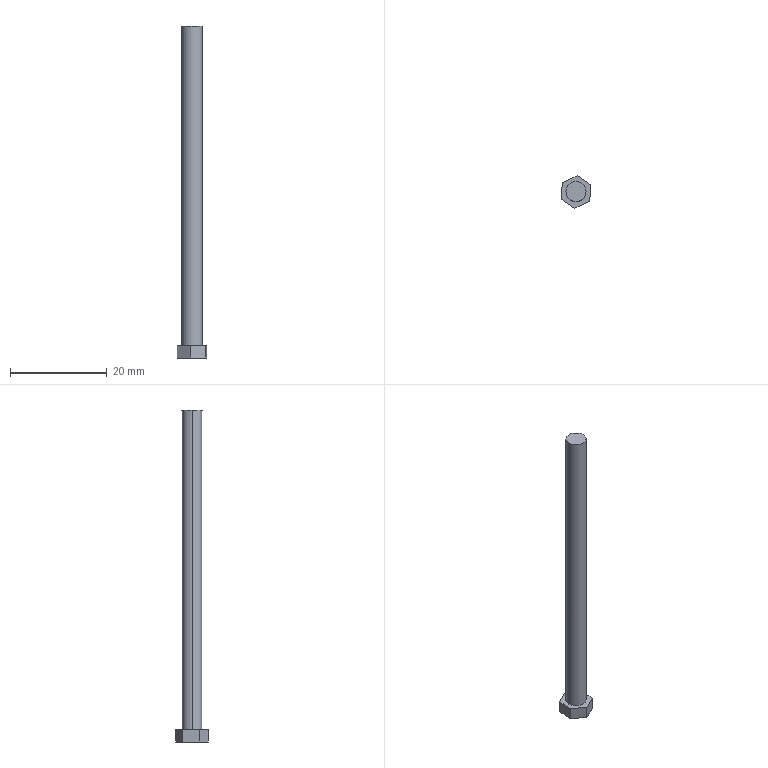Part | SolidWorks | features BaseBody 1 | 1 solid | 11 faces | box 6.123 x 6.803 x 68.58 mm | volume 976.721 mm3 | plane 9 | cylinder 2 | commonest cylinder face diameters 4.166 x2
STEP:
#1=CARTESIAN_POINT('',(2.083,0.,66.04));
#2=VERTEX_POINT('',#1);
#3=CARTESIAN_POINT('',(-2.083,0.,66.04));
#4=VERTEX_POINT('',#3);
#5=CARTESIAN_POINT('',(0.,0.,66.04));
#6=DIRECTION('',(0.,0.,1.));
#7=DIRECTION('',(-1.,0.,0.));
#8=AXIS2_PLACEMENT_3D('',#5,#6,#7);
#9=CIRCLE('',#8,2.083);
#10=EDGE_CURVE('',#2,#4,#9,.T.);
#11=ORIENTED_EDGE('',*,*,#10,.F.);
#12=CARTESIAN_POINT('',(2.083,0.,0.));
#13=VERTEX_POINT('',#12);
#14=CARTESIAN_POINT('',(2.083,0.,66.04));
#15=DIRECTION('',(0.,0.,-1.));
#16=VECTOR('',#15,1000.);
#17=LINE('',#14,#16);
#18=EDGE_CURVE('',#2,#13,#17,.T.);
#19=ORIENTED_EDGE('',*,*,#18,.T.);
#20=CARTESIAN_POINT('',(-2.083,0.,0.));
#21=VERTEX_POINT('',#20);
#22=CARTESIAN_POINT('',(0.,0.,0.));
#23=DIRECTION('',(0.,0.,-1.));
#24=DIRECTION('',(-1.,0.,0.));
#25=AXIS2_PLACEMENT_3D('',#22,#23,#24);
#26=CIRCLE('',#25,2.083);
#27=EDGE_CURVE('',#21,#13,#26,.T.);
#28=ORIENTED_EDGE('',*,*,#27,.F.);
#29=CARTESIAN_POINT('',(-2.083,0.,66.04));
#30=DIRECTION('',(0.,0.,-1.));
#31=VECTOR('',#30,1000.);
#32=LINE('',#29,#31);
#33=EDGE_CURVE('',#4,#21,#32,.T.);
#34=ORIENTED_EDGE('',*,*,#33,.F.);
#35=EDGE_LOOP('',(#11,#19,#28,#34));
#36=FACE_OUTER_BOUND('',#35,.T.);
#37=CARTESIAN_POINT('',(0.,0.,66.04));
#38=DIRECTION('',(0.,0.,-1.));
#39=DIRECTION('',(-1.,0.,0.));
#40=AXIS2_PLACEMENT_3D('',#37,#38,#39);
#41=CYLINDRICAL_SURFACE('',#40,2.083);
#42=ADVANCED_FACE('',(#36),#41,.T.);
#43=ORIENTED_EDGE('',*,*,#18,.F.);
#44=CARTESIAN_POINT('',(0.,0.,66.04));
#45=DIRECTION('',(0.,0.,1.));
#46=DIRECTION('',(-1.,0.,0.));
#47=AXIS2_PLACEMENT_3D('',#44,#45,#46);
#48=CIRCLE('',#47,2.083);
#49=EDGE_CURVE('',#4,#2,#48,.T.);
#50=ORIENTED_EDGE('',*,*,#49,.F.);
#51=ORIENTED_EDGE('',*,*,#33,.T.);
#52=CARTESIAN_POINT('',(0.,0.,0.));
#53=DIRECTION('',(0.,0.,-1.));
#54=DIRECTION('',(-1.,0.,0.));
#55=AXIS2_PLACEMENT_3D('',#52,#53,#54);
#56=CIRCLE('',#55,2.083);
#57=EDGE_CURVE('',#13,#21,#56,.T.);
#58=ORIENTED_EDGE('',*,*,#57,.F.);
#59=EDGE_LOOP('',(#43,#50,#51,#58));
#60=FACE_OUTER_BOUND('',#59,.T.);
#61=CARTESIAN_POINT('',(0.,0.,66.04));
#62=DIRECTION('',(0.,0.,-1.));
#63=DIRECTION('',(-1.,0.,0.));
#64=AXIS2_PLACEMENT_3D('',#61,#62,#63);
#65=CYLINDRICAL_SURFACE('',#64,2.083);
#66=ADVANCED_FACE('',(#60),#65,.T.);
#67=ORIENTED_EDGE('',*,*,#49,.T.);
#68=ORIENTED_EDGE('',*,*,#10,.T.);
#69=EDGE_LOOP('',(#67,#68));
#70=FACE_OUTER_BOUND('',#69,.T.);
#71=CARTESIAN_POINT('',(-2.108,-2.108,66.04));
#72=DIRECTION('',(0.,0.,1.));
#73=DIRECTION('',(1.,0.,0.));
#74=AXIS2_PLACEMENT_3D('',#71,#72,#73);
#75=PLANE('',#74);
#76=ADVANCED_FACE('',(#70),#75,.T.);
#77=ORIENTED_EDGE('',*,*,#27,.T.);
#78=ORIENTED_EDGE('',*,*,#57,.T.);
#79=EDGE_LOOP('',(#77,#78));
#80=FACE_BOUND('',#79,.T.);
#81=CARTESIAN_POINT('',(0.2313,3.401,0.));
#82=VERTEX_POINT('',#81);
#83=CARTESIAN_POINT('',(3.061,1.5,0.));
#84=VERTEX_POINT('',#83);
#85=CARTESIAN_POINT('',(0.2313,3.401,0.));
#86=DIRECTION('',(0.8301,-0.5576,0.));
#87=VECTOR('',#86,1000.);
#88=LINE('',#85,#87);
#89=EDGE_CURVE('',#82,#84,#88,.T.);
#90=ORIENTED_EDGE('',*,*,#89,.F.);
#91=CARTESIAN_POINT('',(-2.83,1.901,0.));
#92=VERTEX_POINT('',#91);
#93=CARTESIAN_POINT('',(-2.83,1.901,0.));
#94=DIRECTION('',(0.898,0.4401,0.));
#95=VECTOR('',#94,1000.);
#96=LINE('',#93,#95);
#97=EDGE_CURVE('',#92,#82,#96,.T.);
#98=ORIENTED_EDGE('',*,*,#97,.F.);
#99=CARTESIAN_POINT('',(-3.061,-1.5,0.));
#100=VERTEX_POINT('',#99);
#101=CARTESIAN_POINT('',(-3.061,-1.5,0.));
#102=DIRECTION('',(0.06785,0.9977,0.));
#103=VECTOR('',#102,1000.);
#104=LINE('',#101,#103);
#105=EDGE_CURVE('',#100,#92,#104,.T.);
#106=ORIENTED_EDGE('',*,*,#105,.F.);
#107=CARTESIAN_POINT('',(-0.2313,-3.401,0.));
#108=VERTEX_POINT('',#107);
#109=CARTESIAN_POINT('',(-0.2313,-3.401,0.));
#110=DIRECTION('',(-0.8301,0.5576,0.));
#111=VECTOR('',#110,1000.);
#112=LINE('',#109,#111);
#113=EDGE_CURVE('',#108,#100,#112,.T.);
#114=ORIENTED_EDGE('',*,*,#113,.F.);
#115=CARTESIAN_POINT('',(2.83,-1.901,0.));
#116=VERTEX_POINT('',#115);
#117=CARTESIAN_POINT('',(2.83,-1.901,0.));
#118=DIRECTION('',(-0.898,-0.4401,0.));
#119=VECTOR('',#118,1000.);
#120=LINE('',#117,#119);
#121=EDGE_CURVE('',#116,#108,#120,.T.);
#122=ORIENTED_EDGE('',*,*,#121,.F.);
#123=CARTESIAN_POINT('',(3.061,1.5,0.));
#124=DIRECTION('',(-0.06785,-0.9977,0.));
#125=VECTOR('',#124,1000.);
#126=LINE('',#123,#125);
#127=EDGE_CURVE('',#84,#116,#126,.T.);
#128=ORIENTED_EDGE('',*,*,#127,.F.);
#129=EDGE_LOOP('',(#90,#98,#106,#114,#122,#128));
#130=FACE_OUTER_BOUND('',#129,.T.);
#131=CARTESIAN_POINT('',(3.098,-3.442,0.));
#132=DIRECTION('',(0.,0.,-1.));
#133=DIRECTION('',(-1.,0.,0.));
#134=AXIS2_PLACEMENT_3D('',#131,#132,#133);
#135=PLANE('',#134);
#136=ADVANCED_FACE('',(#80,#130),#135,.F.);
#137=CARTESIAN_POINT('',(2.83,-1.901,-2.54));
#138=VERTEX_POINT('',#137);
#139=CARTESIAN_POINT('',(2.83,-1.901,-1.27));
#140=DIRECTION('',(0.,0.,1.));
#141=VECTOR('',#140,1000.);
#142=LINE('',#139,#141);
#143=EDGE_CURVE('',#138,#116,#142,.T.);
#144=ORIENTED_EDGE('',*,*,#143,.F.);
#145=CARTESIAN_POINT('',(3.061,1.5,-2.54));
#146=VERTEX_POINT('',#145);
#147=CARTESIAN_POINT('',(2.946,-0.2003,-2.54));
#148=DIRECTION('',(-0.06785,-0.9977,0.));
#149=VECTOR('',#148,1000.);
#150=LINE('',#147,#149);
#151=EDGE_CURVE('',#146,#138,#150,.T.);
#152=ORIENTED_EDGE('',*,*,#151,.F.);
#153=CARTESIAN_POINT('',(3.061,1.5,-1.27));
#154=DIRECTION('',(0.,0.,-1.));
#155=VECTOR('',#154,1000.);
#156=LINE('',#153,#155);
#157=EDGE_CURVE('',#84,#146,#156,.T.);
#158=ORIENTED_EDGE('',*,*,#157,.F.);
#159=ORIENTED_EDGE('',*,*,#127,.T.);
#160=EDGE_LOOP('',(#144,#152,#158,#159));
#161=FACE_OUTER_BOUND('',#160,.T.);
#162=CARTESIAN_POINT('',(3.061,1.5,-2.54));
#163=DIRECTION('',(-0.9977,0.06785,0.));
#164=DIRECTION('',(-0.06785,-0.9977,0.));
#165=AXIS2_PLACEMENT_3D('',#162,#163,#164);
#166=PLANE('',#165);
#167=ADVANCED_FACE('',(#161),#166,.F.);
#168=ORIENTED_EDGE('',*,*,#157,.T.);
#169=CARTESIAN_POINT('',(0.2313,3.401,-2.54));
#170=VERTEX_POINT('',#169);
#171=CARTESIAN_POINT('',(1.646,2.451,-2.54));
#172=DIRECTION('',(0.8301,-0.5576,0.));
#173=VECTOR('',#172,1000.);
#174=LINE('',#171,#173);
#175=EDGE_CURVE('',#170,#146,#174,.T.);
#176=ORIENTED_EDGE('',*,*,#175,.F.);
#177=CARTESIAN_POINT('',(0.2313,3.401,-1.27));
#178=DIRECTION('',(0.,0.,-1.));
#179=VECTOR('',#178,1000.);
#180=LINE('',#177,#179);
#181=EDGE_CURVE('',#82,#170,#180,.T.);
#182=ORIENTED_EDGE('',*,*,#181,.F.);
#183=ORIENTED_EDGE('',*,*,#89,.T.);
#184=EDGE_LOOP('',(#168,#176,#182,#183));
#185=FACE_OUTER_BOUND('',#184,.T.);
#186=CARTESIAN_POINT('',(0.2313,3.401,-2.54));
#187=DIRECTION('',(-0.5576,-0.8301,0.));
#188=DIRECTION('',(0.8301,-0.5576,0.));
#189=AXIS2_PLACEMENT_3D('',#186,#187,#188);
#190=PLANE('',#189);
#191=ADVANCED_FACE('',(#185),#190,.F.);
#192=ORIENTED_EDGE('',*,*,#181,.T.);
#193=CARTESIAN_POINT('',(-2.83,1.901,-2.54));
#194=VERTEX_POINT('',#193);
#195=CARTESIAN_POINT('',(-1.299,2.651,-2.54));
#196=DIRECTION('',(0.898,0.4401,0.));
#197=VECTOR('',#196,1000.);
#198=LINE('',#195,#197);
#199=EDGE_CURVE('',#194,#170,#198,.T.);
#200=ORIENTED_EDGE('',*,*,#199,.F.);
#201=CARTESIAN_POINT('',(-2.83,1.901,-1.27));
#202=DIRECTION('',(0.,0.,-1.));
#203=VECTOR('',#202,1000.);
#204=LINE('',#201,#203);
#205=EDGE_CURVE('',#92,#194,#204,.T.);
#206=ORIENTED_EDGE('',*,*,#205,.F.);
#207=ORIENTED_EDGE('',*,*,#97,.T.);
#208=EDGE_LOOP('',(#192,#200,#206,#207));
#209=FACE_OUTER_BOUND('',#208,.T.);
#210=CARTESIAN_POINT('',(-2.83,1.901,-2.54));
#211=DIRECTION('',(0.4401,-0.898,0.));
#212=DIRECTION('',(0.898,0.4401,0.));
#213=AXIS2_PLACEMENT_3D('',#210,#211,#212);
#214=PLANE('',#213);
#215=ADVANCED_FACE('',(#209),#214,.F.);
#216=ORIENTED_EDGE('',*,*,#205,.T.);
#217=CARTESIAN_POINT('',(-3.061,-1.5,-2.54));
#218=VERTEX_POINT('',#217);
#219=CARTESIAN_POINT('',(-2.946,0.2003,-2.54));
#220=DIRECTION('',(0.06785,0.9977,0.));
#221=VECTOR('',#220,1000.);
#222=LINE('',#219,#221);
#223=EDGE_CURVE('',#218,#194,#222,.T.);
#224=ORIENTED_EDGE('',*,*,#223,.F.);
#225=CARTESIAN_POINT('',(-3.061,-1.5,-1.27));
#226=DIRECTION('',(0.,0.,-1.));
#227=VECTOR('',#226,1000.);
#228=LINE('',#225,#227);
#229=EDGE_CURVE('',#100,#218,#228,.T.);
#230=ORIENTED_EDGE('',*,*,#229,.F.);
#231=ORIENTED_EDGE('',*,*,#105,.T.);
#232=EDGE_LOOP('',(#216,#224,#230,#231));
#233=FACE_OUTER_BOUND('',#232,.T.);
#234=CARTESIAN_POINT('',(-3.061,-1.5,-2.54));
#235=DIRECTION('',(0.9977,-0.06785,0.));
#236=DIRECTION('',(0.06785,0.9977,0.));
#237=AXIS2_PLACEMENT_3D('',#234,#235,#236);
#238=PLANE('',#237);
#239=ADVANCED_FACE('',(#233),#238,.F.);
#240=ORIENTED_EDGE('',*,*,#229,.T.);
#241=CARTESIAN_POINT('',(-0.2313,-3.401,-2.54));
#242=VERTEX_POINT('',#241);
#243=CARTESIAN_POINT('',(-1.646,-2.451,-2.54));
#244=DIRECTION('',(-0.8301,0.5576,0.));
#245=VECTOR('',#244,1000.);
#246=LINE('',#243,#245);
#247=EDGE_CURVE('',#242,#218,#246,.T.);
#248=ORIENTED_EDGE('',*,*,#247,.F.);
#249=CARTESIAN_POINT('',(-0.2313,-3.401,-1.27));
#250=DIRECTION('',(0.,0.,-1.));
#251=VECTOR('',#250,1000.);
#252=LINE('',#249,#251);
#253=EDGE_CURVE('',#108,#242,#252,.T.);
#254=ORIENTED_EDGE('',*,*,#253,.F.);
#255=ORIENTED_EDGE('',*,*,#113,.T.);
#256=EDGE_LOOP('',(#240,#248,#254,#255));
#257=FACE_OUTER_BOUND('',#256,.T.);
#258=CARTESIAN_POINT('',(-0.2313,-3.401,-2.54));
#259=DIRECTION('',(0.5576,0.8301,0.));
#260=DIRECTION('',(-0.8301,0.5576,0.));
#261=AXIS2_PLACEMENT_3D('',#258,#259,#260);
#262=PLANE('',#261);
#263=ADVANCED_FACE('',(#257),#262,.F.);
#264=ORIENTED_EDGE('',*,*,#253,.T.);
#265=CARTESIAN_POINT('',(1.299,-2.651,-2.54));
#266=DIRECTION('',(-0.898,-0.4401,0.));
#267=VECTOR('',#266,1000.);
#268=LINE('',#265,#267);
#269=EDGE_CURVE('',#138,#242,#268,.T.);
#270=ORIENTED_EDGE('',*,*,#269,.F.);
#271=ORIENTED_EDGE('',*,*,#143,.T.);
#272=ORIENTED_EDGE('',*,*,#121,.T.);
#273=EDGE_LOOP('',(#264,#270,#271,#272));
#274=FACE_OUTER_BOUND('',#273,.T.);
#275=CARTESIAN_POINT('',(2.83,-1.901,-2.54));
#276=DIRECTION('',(-0.4401,0.898,0.));
#277=DIRECTION('',(-0.898,-0.4401,0.));
#278=AXIS2_PLACEMENT_3D('',#275,#276,#277);
#279=PLANE('',#278);
#280=ADVANCED_FACE('',(#274),#279,.F.);
#281=ORIENTED_EDGE('',*,*,#199,.T.);
#282=ORIENTED_EDGE('',*,*,#175,.T.);
#283=ORIENTED_EDGE('',*,*,#151,.T.);
#284=ORIENTED_EDGE('',*,*,#269,.T.);
#285=ORIENTED_EDGE('',*,*,#247,.T.);
#286=ORIENTED_EDGE('',*,*,#223,.T.);
#287=EDGE_LOOP('',(#281,#282,#283,#284,#285,#286));
#288=FACE_OUTER_BOUND('',#287,.T.);
#289=CARTESIAN_POINT('',(3.061,-3.401,-2.54));
#290=DIRECTION('',(0.,0.,-1.));
#291=DIRECTION('',(-1.,0.,0.));
#292=AXIS2_PLACEMENT_3D('',#289,#290,#291);
#293=PLANE('',#292);
#294=ADVANCED_FACE('',(#288),#293,.T.);
#295=CLOSED_SHELL('',(#42,#66,#76,#136,#167,#191,#215,#239,#263,#280,#294));
#296=MANIFOLD_SOLID_BREP('',#295);
#297=CARTESIAN_POINT('',(0.,0.,0.));
#298=DIRECTION('',(0.,0.,1.));
#299=DIRECTION('',(1.,0.,0.));
#300=AXIS2_PLACEMENT_3D('',#297,#298,#299);
#301=(LENGTH_UNIT()NAMED_UNIT(*)SI_UNIT(.MILLI.,.METRE.));
#302=UNCERTAINTY_MEASURE_WITH_UNIT(LENGTH_MEASURE(0.00001),#301,'','');
#303=(NAMED_UNIT(*)PLANE_ANGLE_UNIT()SI_UNIT($,.RADIAN.));
#304=(NAMED_UNIT(*)SI_UNIT($,.STERADIAN.)SOLID_ANGLE_UNIT());
#305=(GEOMETRIC_REPRESENTATION_CONTEXT(3)GLOBAL_UNCERTAINTY_ASSIGNED_CONTEXT((#302))GLOBAL_UNIT_ASSIGNED_CONTEXT((#301,#303,#304))REPRESENTATION_CONTEXT('',''));
#306=ADVANCED_BREP_SHAPE_REPRESENTATION('',(#296,#300),#305);